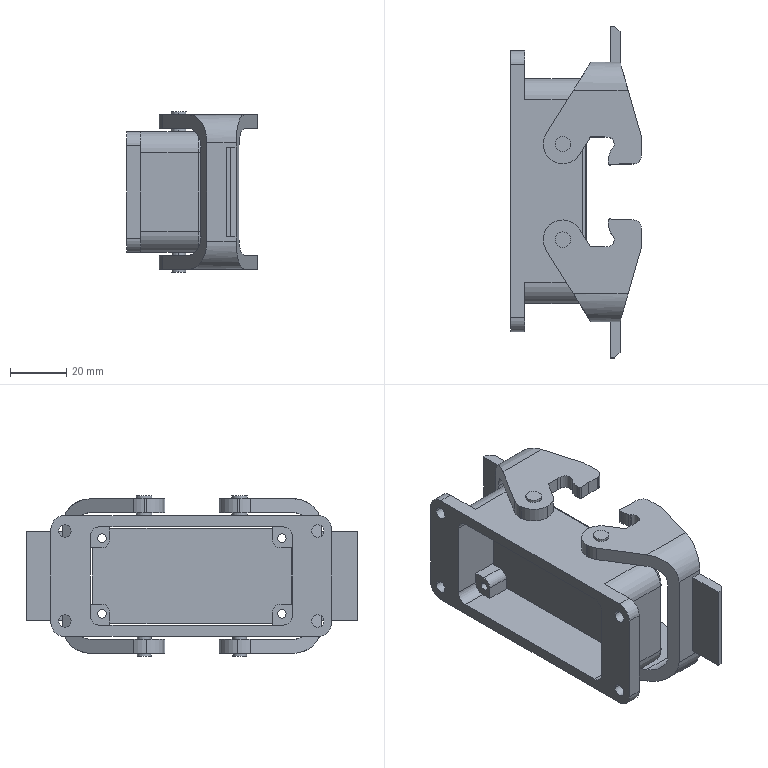Part | STEP file | 4-20.sldasm-Part-11 | 1 solid | 260 faces | box 46.6 x 118.128 x 57 mm | volume 74877 mm3 | cylinder 126 | plane 126 | torus 8 | commonest cylinder face diameters 2 x20 7 x12 3 x8 3.3 x8 4.4 x8 5.5 x8